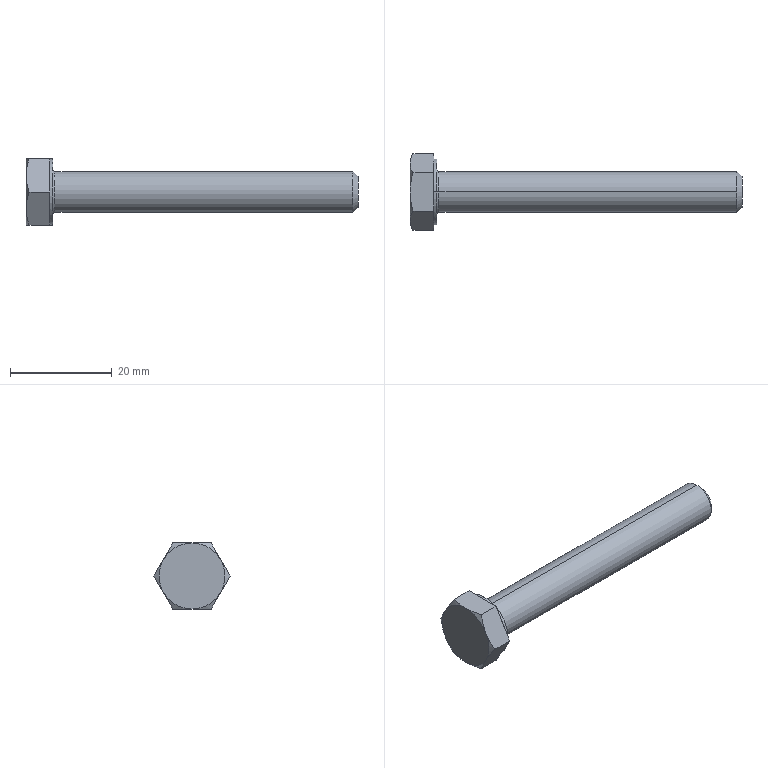Part | SolidWorks | features RevCut 4, Chamfer 1, Extrusion 1, Fillet 1, LPattern 1, Revolution 1 | 1 solid | 29 faces | box 65.3 x 15.011 x 13 mm | volume 3770 mm3 | plane 15 | cone 8 | cylinder 4 | torus 2 | commonest cylinder face diameters 8 x2 13 x2
STEP:
#1=CARTESIAN_POINT('',(5.7,0.,4.));
#2=VERTEX_POINT('',#1);
#3=CARTESIAN_POINT('',(5.7,0.,-4.));
#4=VERTEX_POINT('',#3);
#5=CARTESIAN_POINT('',(5.7,0.,0.));
#6=DIRECTION('',(1.,0.,0.));
#7=DIRECTION('',(0.,0.,-1.));
#8=AXIS2_PLACEMENT_3D('',#5,#6,#7);
#9=CIRCLE('',#8,4.);
#10=EDGE_CURVE('',#2,#4,#9,.T.);
#11=ORIENTED_EDGE('',*,*,#10,.F.);
#12=CARTESIAN_POINT('',(5.3,0.,4.4));
#13=VERTEX_POINT('',#12);
#14=CARTESIAN_POINT('',(5.7,0.,4.4));
#15=DIRECTION('',(0.,1.,0.));
#16=DIRECTION('',(0.,0.,1.));
#17=AXIS2_PLACEMENT_3D('',#14,#15,#16);
#18=CIRCLE('',#17,0.4);
#19=EDGE_CURVE('',#2,#13,#18,.T.);
#20=ORIENTED_EDGE('',*,*,#19,.T.);
#21=CARTESIAN_POINT('',(5.3,0.,-4.4));
#22=VERTEX_POINT('',#21);
#23=CARTESIAN_POINT('',(5.3,0.,0.));
#24=DIRECTION('',(-1.,0.,0.));
#25=DIRECTION('',(0.,0.,-1.));
#26=AXIS2_PLACEMENT_3D('',#23,#24,#25);
#27=CIRCLE('',#26,4.4);
#28=EDGE_CURVE('',#22,#13,#27,.T.);
#29=ORIENTED_EDGE('',*,*,#28,.F.);
#30=CARTESIAN_POINT('',(5.7,0.,-4.4));
#31=DIRECTION('',(0.,-1.,0.));
#32=DIRECTION('',(0.,0.,-1.));
#33=AXIS2_PLACEMENT_3D('',#30,#31,#32);
#34=CIRCLE('',#33,0.4);
#35=EDGE_CURVE('',#4,#22,#34,.T.);
#36=ORIENTED_EDGE('',*,*,#35,.F.);
#37=EDGE_LOOP('',(#11,#20,#29,#36));
#38=FACE_OUTER_BOUND('',#37,.T.);
#39=CARTESIAN_POINT('',(5.7,0.,0.));
#40=DIRECTION('',(1.,0.,0.));
#41=DIRECTION('',(0.,0.,-1.));
#42=AXIS2_PLACEMENT_3D('',#39,#40,#41);
#43=TOROIDAL_SURFACE('',#42,4.4,0.4);
#44=ADVANCED_FACE('',(#38),#43,.F.);
#45=CARTESIAN_POINT('',(65.3,0.,-3.));
#46=VERTEX_POINT('',#45);
#47=CARTESIAN_POINT('',(65.3,0.,3.));
#48=VERTEX_POINT('',#47);
#49=CARTESIAN_POINT('',(65.3,0.,0.));
#50=DIRECTION('',(1.,0.,0.));
#51=DIRECTION('',(0.,0.,1.));
#52=AXIS2_PLACEMENT_3D('',#49,#50,#51);
#53=CIRCLE('',#52,3.);
#54=EDGE_CURVE('',#46,#48,#53,.T.);
#55=ORIENTED_EDGE('',*,*,#54,.F.);
#56=CARTESIAN_POINT('',(64.3,0.,-4.));
#57=VERTEX_POINT('',#56);
#58=CARTESIAN_POINT('',(64.3,0.,-4.));
#59=DIRECTION('',(-0.7071,0.,-0.7071));
#60=VECTOR('',#59,1000.);
#61=LINE('',#58,#60);
#62=EDGE_CURVE('',#46,#57,#61,.T.);
#63=ORIENTED_EDGE('',*,*,#62,.T.);
#64=CARTESIAN_POINT('',(64.3,0.,4.));
#65=VERTEX_POINT('',#64);
#66=CARTESIAN_POINT('',(64.3,0.,0.));
#67=DIRECTION('',(-1.,0.,0.));
#68=DIRECTION('',(0.,0.,1.));
#69=AXIS2_PLACEMENT_3D('',#66,#67,#68);
#70=CIRCLE('',#69,4.);
#71=EDGE_CURVE('',#65,#57,#70,.T.);
#72=ORIENTED_EDGE('',*,*,#71,.F.);
#73=CARTESIAN_POINT('',(64.3,0.,4.));
#74=DIRECTION('',(-0.7071,0.,0.7071));
#75=VECTOR('',#74,1000.);
#76=LINE('',#73,#75);
#77=EDGE_CURVE('',#48,#65,#76,.T.);
#78=ORIENTED_EDGE('',*,*,#77,.F.);
#79=EDGE_LOOP('',(#55,#63,#72,#78));
#80=FACE_OUTER_BOUND('',#79,.T.);
#81=CARTESIAN_POINT('',(64.3,0.,0.));
#82=DIRECTION('',(-1.,0.,0.));
#83=DIRECTION('',(0.,0.,1.));
#84=AXIS2_PLACEMENT_3D('',#81,#82,#83);
#85=CONICAL_SURFACE('',#84,4.,0.7854);
#86=ADVANCED_FACE('',(#80),#85,.T.);
#87=ORIENTED_EDGE('',*,*,#71,.T.);
#88=CARTESIAN_POINT('',(0.,0.,-4.));
#89=DIRECTION('',(-1.,0.,0.));
#90=VECTOR('',#89,1000.);
#91=LINE('',#88,#90);
#92=EDGE_CURVE('',#57,#4,#91,.T.);
#93=ORIENTED_EDGE('',*,*,#92,.T.);
#94=CARTESIAN_POINT('',(5.7,0.,0.));
#95=DIRECTION('',(1.,0.,0.));
#96=DIRECTION('',(0.,0.,-1.));
#97=AXIS2_PLACEMENT_3D('',#94,#95,#96);
#98=CIRCLE('',#97,4.);
#99=EDGE_CURVE('',#4,#2,#98,.T.);
#100=ORIENTED_EDGE('',*,*,#99,.T.);
#101=CARTESIAN_POINT('',(0.,0.,4.));
#102=DIRECTION('',(-1.,0.,0.));
#103=VECTOR('',#102,1000.);
#104=LINE('',#101,#103);
#105=EDGE_CURVE('',#65,#2,#104,.T.);
#106=ORIENTED_EDGE('',*,*,#105,.F.);
#107=EDGE_LOOP('',(#87,#93,#100,#106));
#108=FACE_OUTER_BOUND('',#107,.T.);
#109=CARTESIAN_POINT('',(0.,0.,0.));
#110=DIRECTION('',(-1.,0.,0.));
#111=DIRECTION('',(0.,0.,1.));
#112=AXIS2_PLACEMENT_3D('',#109,#110,#111);
#113=CYLINDRICAL_SURFACE('',#112,4.);
#114=ADVANCED_FACE('',(#108),#113,.T.);
#115=CARTESIAN_POINT('',(5.3,0.,-6.5));
#116=VERTEX_POINT('',#115);
#117=CARTESIAN_POINT('',(5.3,0.,6.5));
#118=VERTEX_POINT('',#117);
#119=CARTESIAN_POINT('',(5.3,0.,0.));
#120=DIRECTION('',(1.,0.,0.));
#121=DIRECTION('',(0.,0.,-1.));
#122=AXIS2_PLACEMENT_3D('',#119,#120,#121);
#123=CIRCLE('',#122,6.5);
#124=EDGE_CURVE('',#116,#118,#123,.T.);
#125=ORIENTED_EDGE('',*,*,#124,.F.);
#126=CARTESIAN_POINT('',(4.7,0.,-6.5));
#127=VERTEX_POINT('',#126);
#128=CARTESIAN_POINT('',(0.,0.,-6.5));
#129=DIRECTION('',(-1.,0.,0.));
#130=VECTOR('',#129,1000.);
#131=LINE('',#128,#130);
#132=EDGE_CURVE('',#116,#127,#131,.T.);
#133=ORIENTED_EDGE('',*,*,#132,.T.);
#134=CARTESIAN_POINT('',(4.7,5.629,-3.25));
#135=VERTEX_POINT('',#134);
#136=CARTESIAN_POINT('',(4.7,0.,0.));
#137=DIRECTION('',(-1.,0.,0.));
#138=DIRECTION('',(0.,0.,1.));
#139=AXIS2_PLACEMENT_3D('',#136,#137,#138);
#140=CIRCLE('',#139,6.5);
#141=EDGE_CURVE('',#135,#127,#140,.T.);
#142=ORIENTED_EDGE('',*,*,#141,.F.);
#143=CARTESIAN_POINT('',(4.7,5.629,3.25));
#144=VERTEX_POINT('',#143);
#145=CARTESIAN_POINT('',(4.7,0.,0.));
#146=DIRECTION('',(-1.,0.,0.));
#147=DIRECTION('',(0.,0.,1.));
#148=AXIS2_PLACEMENT_3D('',#145,#146,#147);
#149=CIRCLE('',#148,6.5);
#150=EDGE_CURVE('',#144,#135,#149,.T.);
#151=ORIENTED_EDGE('',*,*,#150,.F.);
#152=CARTESIAN_POINT('',(4.7,0.,6.5));
#153=VERTEX_POINT('',#152);
#154=CARTESIAN_POINT('',(4.7,0.,0.));
#155=DIRECTION('',(-1.,0.,0.));
#156=DIRECTION('',(0.,0.,1.));
#157=AXIS2_PLACEMENT_3D('',#154,#155,#156);
#158=CIRCLE('',#157,6.5);
#159=EDGE_CURVE('',#153,#144,#158,.T.);
#160=ORIENTED_EDGE('',*,*,#159,.F.);
#161=CARTESIAN_POINT('',(0.,0.,6.5));
#162=DIRECTION('',(-1.,0.,0.));
#163=VECTOR('',#162,1000.);
#164=LINE('',#161,#163);
#165=EDGE_CURVE('',#118,#153,#164,.T.);
#166=ORIENTED_EDGE('',*,*,#165,.F.);
#167=EDGE_LOOP('',(#125,#133,#142,#151,#160,#166));
#168=FACE_OUTER_BOUND('',#167,.T.);
#169=CARTESIAN_POINT('',(0.,0.,0.));
#170=DIRECTION('',(-1.,0.,0.));
#171=DIRECTION('',(0.,0.,1.));
#172=AXIS2_PLACEMENT_3D('',#169,#170,#171);
#173=CYLINDRICAL_SURFACE('',#172,6.5);
#174=ADVANCED_FACE('',(#168),#173,.T.);
#175=CARTESIAN_POINT('',(4.7,3.753,-6.5));
#176=VERTEX_POINT('',#175);
#177=CARTESIAN_POINT('',(4.7,3.753,-6.5));
#178=DIRECTION('',(0.,0.5,0.866));
#179=VECTOR('',#178,1000.);
#180=LINE('',#177,#179);
#181=EDGE_CURVE('',#176,#135,#180,.T.);
#182=ORIENTED_EDGE('',*,*,#181,.F.);
#183=CARTESIAN_POINT('',(0.5806,3.753,-6.5));
#184=VERTEX_POINT('',#183);
#185=CARTESIAN_POINT('',(5.3,3.753,-6.5));
#186=DIRECTION('',(-1.,0.,0.));
#187=VECTOR('',#186,1000.);
#188=LINE('',#185,#187);
#189=EDGE_CURVE('',#176,#184,#188,.T.);
#190=ORIENTED_EDGE('',*,*,#189,.T.);
#191=CARTESIAN_POINT('',(0.,5.629,-3.25));
#192=VERTEX_POINT('',#191);
#193=CARTESIAN_POINT('',(0.,5.629,-3.25));
#194=CARTESIAN_POINT('',(0.,5.47,-3.526));
#195=CARTESIAN_POINT('',(0.01372,5.31,-3.803));
#196=CARTESIAN_POINT('',(0.06683,4.994,-4.351));
#197=CARTESIAN_POINT('',(0.1062,4.836,-4.623));
#198=CARTESIAN_POINT('',(0.2578,4.368,-5.435));
#199=CARTESIAN_POINT('',(0.4038,4.059,-5.97));
#200=CARTESIAN_POINT('',(0.5806,3.753,-6.5));
#201=B_SPLINE_CURVE_WITH_KNOTS('',3,(#193,#194,#195,#196,#197,#198,#199,#200),.UNSPECIFIED.,.F.,.F.,(4,2,2,4),(0.003797,0.004743,0.005689,0.00758),.UNSPECIFIED.);
#202=EDGE_CURVE('',#192,#184,#201,.T.);
#203=ORIENTED_EDGE('',*,*,#202,.F.);
#204=CARTESIAN_POINT('',(0.5806,7.506,0.));
#205=VERTEX_POINT('',#204);
#206=CARTESIAN_POINT('',(0.5806,7.506,0.));
#207=CARTESIAN_POINT('',(0.4033,7.199,-0.5317));
#208=CARTESIAN_POINT('',(0.2573,6.889,-1.067));
#209=CARTESIAN_POINT('',(0.05533,6.265,-2.149));
#210=CARTESIAN_POINT('',(0.,5.949,-2.696));
#211=CARTESIAN_POINT('',(0.,5.629,-3.25));
#212=B_SPLINE_CURVE_WITH_KNOTS('',3,(#206,#207,#208,#209,#210,#211),.UNSPECIFIED.,.F.,.F.,(4,2,4),(0.000000238,0.001899,0.003797),.UNSPECIFIED.);
#213=EDGE_CURVE('',#205,#192,#212,.T.);
#214=ORIENTED_EDGE('',*,*,#213,.F.);
#215=CARTESIAN_POINT('',(4.7,7.506,0.));
#216=VERTEX_POINT('',#215);
#217=CARTESIAN_POINT('',(5.3,7.506,0.));
#218=DIRECTION('',(-1.,0.,0.));
#219=VECTOR('',#218,1000.);
#220=LINE('',#217,#219);
#221=EDGE_CURVE('',#216,#205,#220,.T.);
#222=ORIENTED_EDGE('',*,*,#221,.F.);
#223=CARTESIAN_POINT('',(4.7,3.753,-6.5));
#224=DIRECTION('',(0.,0.5,0.866));
#225=VECTOR('',#224,1000.);
#226=LINE('',#223,#225);
#227=EDGE_CURVE('',#135,#216,#226,.T.);
#228=ORIENTED_EDGE('',*,*,#227,.F.);
#229=EDGE_LOOP('',(#182,#190,#203,#214,#222,#228));
#230=FACE_OUTER_BOUND('',#229,.T.);
#231=CARTESIAN_POINT('',(5.3,3.753,-6.5));
#232=DIRECTION('',(0.,-0.866,0.5));
#233=DIRECTION('',(0.,-0.5,-0.866));
#234=AXIS2_PLACEMENT_3D('',#231,#232,#233);
#235=PLANE('',#234);
#236=ADVANCED_FACE('',(#230),#235,.F.);
#237=CARTESIAN_POINT('',(4.7,7.506,0.));
#238=DIRECTION('',(0.,-0.5,0.866));
#239=VECTOR('',#238,1000.);
#240=LINE('',#237,#239);
#241=EDGE_CURVE('',#216,#144,#240,.T.);
#242=ORIENTED_EDGE('',*,*,#241,.F.);
#243=ORIENTED_EDGE('',*,*,#221,.T.);
#244=CARTESIAN_POINT('',(0.,5.629,3.25));
#245=VERTEX_POINT('',#244);
#246=CARTESIAN_POINT('',(0.,5.629,3.25));
#247=CARTESIAN_POINT('',(0.,5.788,2.974));
#248=CARTESIAN_POINT('',(0.01372,5.948,2.697));
#249=CARTESIAN_POINT('',(0.06683,6.265,2.149));
#250=CARTESIAN_POINT('',(0.1062,6.422,1.877));
#251=CARTESIAN_POINT('',(0.2578,6.891,1.065));
#252=CARTESIAN_POINT('',(0.4038,7.199,0.5303));
#253=CARTESIAN_POINT('',(0.5806,7.506,0.));
#254=B_SPLINE_CURVE_WITH_KNOTS('',3,(#246,#247,#248,#249,#250,#251,#252,#253),.UNSPECIFIED.,.F.,.F.,(4,2,2,4),(0.003797,0.004743,0.005689,0.00758),.UNSPECIFIED.);
#255=EDGE_CURVE('',#245,#205,#254,.T.);
#256=ORIENTED_EDGE('',*,*,#255,.F.);
#257=CARTESIAN_POINT('',(0.5806,3.753,6.5));
#258=VERTEX_POINT('',#257);
#259=CARTESIAN_POINT('',(0.5806,3.753,6.5));
#260=CARTESIAN_POINT('',(0.4033,4.06,5.968));
#261=CARTESIAN_POINT('',(0.2573,4.369,5.433));
#262=CARTESIAN_POINT('',(0.05533,4.994,4.351));
#263=CARTESIAN_POINT('',(0.,5.309,3.804));
#264=CARTESIAN_POINT('',(0.,5.629,3.25));
#265=B_SPLINE_CURVE_WITH_KNOTS('',3,(#259,#260,#261,#262,#263,#264),.UNSPECIFIED.,.F.,.F.,(4,2,4),(0.000000238,0.001899,0.003797),.UNSPECIFIED.);
#266=EDGE_CURVE('',#258,#245,#265,.T.);
#267=ORIENTED_EDGE('',*,*,#266,.F.);
#268=CARTESIAN_POINT('',(4.7,3.753,6.5));
#269=VERTEX_POINT('',#268);
#270=CARTESIAN_POINT('',(5.3,3.753,6.5));
#271=DIRECTION('',(-1.,0.,0.));
#272=VECTOR('',#271,1000.);
#273=LINE('',#270,#272);
#274=EDGE_CURVE('',#269,#258,#273,.T.);
#275=ORIENTED_EDGE('',*,*,#274,.F.);
#276=CARTESIAN_POINT('',(4.7,7.506,0.));
#277=DIRECTION('',(0.,-0.5,0.866));
#278=VECTOR('',#277,1000.);
#279=LINE('',#276,#278);
#280=EDGE_CURVE('',#144,#269,#279,.T.);
#281=ORIENTED_EDGE('',*,*,#280,.F.);
#282=EDGE_LOOP('',(#242,#243,#256,#267,#275,#281));
#283=FACE_OUTER_BOUND('',#282,.T.);
#284=CARTESIAN_POINT('',(5.3,7.506,0.));
#285=DIRECTION('',(0.,-0.866,-0.5));
#286=DIRECTION('',(0.,0.5,-0.866));
#287=AXIS2_PLACEMENT_3D('',#284,#285,#286);
#288=PLANE('',#287);
#289=ADVANCED_FACE('',(#283),#288,.F.);
#290=CARTESIAN_POINT('',(4.7,3.753,6.5));
#291=DIRECTION('',(0.,-1.,0.));
#292=VECTOR('',#291,1000.);
#293=LINE('',#290,#292);
#294=EDGE_CURVE('',#269,#153,#293,.T.);
#295=ORIENTED_EDGE('',*,*,#294,.F.);
#296=ORIENTED_EDGE('',*,*,#274,.T.);
#297=CARTESIAN_POINT('',(0.,0.,6.5));
#298=VERTEX_POINT('',#297);
#299=CARTESIAN_POINT('',(0.,0.,6.5));
#300=CARTESIAN_POINT('',(0.,0.6351,6.5));
#301=CARTESIAN_POINT('',(0.05613,1.279,6.5));
#302=CARTESIAN_POINT('',(0.2595,2.531,6.5));
#303=CARTESIAN_POINT('',(0.4054,3.146,6.5));
#304=CARTESIAN_POINT('',(0.5806,3.753,6.5));
#305=B_SPLINE_CURVE_WITH_KNOTS('',3,(#299,#300,#301,#302,#303,#304),.UNSPECIFIED.,.F.,.F.,(4,2,4),(0.01067,0.01257,0.01447),.UNSPECIFIED.);
#306=EDGE_CURVE('',#298,#258,#305,.T.);
#307=ORIENTED_EDGE('',*,*,#306,.F.);
#308=CARTESIAN_POINT('',(0.5806,-3.753,6.5));
#309=VERTEX_POINT('',#308);
#310=CARTESIAN_POINT('',(0.5806,-3.753,6.5));
#311=CARTESIAN_POINT('',(0.4042,-3.142,6.5));
#312=CARTESIAN_POINT('',(0.2565,-2.517,6.5));
#313=CARTESIAN_POINT('',(0.05459,-1.265,6.5));
#314=CARTESIAN_POINT('',(0.,-0.6347,6.5));
#315=CARTESIAN_POINT('',(0.,0.,6.5));
#316=B_SPLINE_CURVE_WITH_KNOTS('',3,(#310,#311,#312,#313,#314,#315),.UNSPECIFIED.,.F.,.F.,(4,2,4),(0.006874,0.008773,0.01067),.UNSPECIFIED.);
#317=EDGE_CURVE('',#309,#298,#316,.T.);
#318=ORIENTED_EDGE('',*,*,#317,.F.);
#319=CARTESIAN_POINT('',(4.7,-3.753,6.5));
#320=VERTEX_POINT('',#319);
#321=CARTESIAN_POINT('',(5.3,-3.753,6.5));
#322=DIRECTION('',(-1.,0.,0.));
#323=VECTOR('',#322,1000.);
#324=LINE('',#321,#323);
#325=EDGE_CURVE('',#320,#309,#324,.T.);
#326=ORIENTED_EDGE('',*,*,#325,.F.);
#327=CARTESIAN_POINT('',(4.7,3.753,6.5));
#328=DIRECTION('',(0.,-1.,0.));
#329=VECTOR('',#328,1000.);
#330=LINE('',#327,#329);
#331=EDGE_CURVE('',#153,#320,#330,.T.);
#332=ORIENTED_EDGE('',*,*,#331,.F.);
#333=EDGE_LOOP('',(#295,#296,#307,#318,#326,#332));
#334=FACE_OUTER_BOUND('',#333,.T.);
#335=CARTESIAN_POINT('',(5.3,3.753,6.5));
#336=DIRECTION('',(0.,0.,-1.));
#337=DIRECTION('',(0.,1.,0.));
#338=AXIS2_PLACEMENT_3D('',#335,#336,#337);
#339=PLANE('',#338);
#340=ADVANCED_FACE('',(#334),#339,.F.);
#341=CARTESIAN_POINT('',(4.7,-5.629,3.25));
#342=VERTEX_POINT('',#341);
#343=CARTESIAN_POINT('',(4.7,-7.506,0.));
#344=DIRECTION('',(0.,-0.5,-0.866));
#345=VECTOR('',#344,1000.);
#346=LINE('',#343,#345);
#347=EDGE_CURVE('',#320,#342,#346,.T.);
#348=ORIENTED_EDGE('',*,*,#347,.F.);
#349=ORIENTED_EDGE('',*,*,#325,.T.);
#350=CARTESIAN_POINT('',(0.,-5.629,3.25));
#351=VERTEX_POINT('',#350);
#352=CARTESIAN_POINT('',(0.,-5.629,3.25));
#353=CARTESIAN_POINT('',(0.,-5.47,3.526));
#354=CARTESIAN_POINT('',(0.01372,-5.31,3.803));
#355=CARTESIAN_POINT('',(0.06683,-4.994,4.351));
#356=CARTESIAN_POINT('',(0.1062,-4.836,4.623));
#357=CARTESIAN_POINT('',(0.2578,-4.368,5.435));
#358=CARTESIAN_POINT('',(0.4038,-4.059,5.97));
#359=CARTESIAN_POINT('',(0.5806,-3.753,6.5));
#360=B_SPLINE_CURVE_WITH_KNOTS('',3,(#352,#353,#354,#355,#356,#357,#358,#359),.UNSPECIFIED.,.F.,.F.,(4,2,2,4),(0.003797,0.004743,0.005689,0.00758),.UNSPECIFIED.);
#361=EDGE_CURVE('',#351,#309,#360,.T.);
#362=ORIENTED_EDGE('',*,*,#361,.F.);
#363=CARTESIAN_POINT('',(0.5806,-7.506,0.));
#364=VERTEX_POINT('',#363);
#365=CARTESIAN_POINT('',(0.5806,-7.506,0.));
#366=CARTESIAN_POINT('',(0.4033,-7.199,0.5317));
#367=CARTESIAN_POINT('',(0.2573,-6.889,1.067));
#368=CARTESIAN_POINT('',(0.05533,-6.265,2.149));
#369=CARTESIAN_POINT('',(0.,-5.949,2.696));
#370=CARTESIAN_POINT('',(0.,-5.629,3.25));
#371=B_SPLINE_CURVE_WITH_KNOTS('',3,(#365,#366,#367,#368,#369,#370),.UNSPECIFIED.,.F.,.F.,(4,2,4),(0.000000238,0.001899,0.003797),.UNSPECIFIED.);
#372=EDGE_CURVE('',#364,#351,#371,.T.);
#373=ORIENTED_EDGE('',*,*,#372,.F.);
#374=CARTESIAN_POINT('',(4.7,-7.506,0.));
#375=VERTEX_POINT('',#374);
#376=CARTESIAN_POINT('',(5.3,-7.506,0.));
#377=DIRECTION('',(-1.,0.,0.));
#378=VECTOR('',#377,1000.);
#379=LINE('',#376,#378);
#380=EDGE_CURVE('',#375,#364,#379,.T.);
#381=ORIENTED_EDGE('',*,*,#380,.F.);
#382=CARTESIAN_POINT('',(4.7,-7.506,0.));
#383=DIRECTION('',(0.,-0.5,-0.866));
#384=VECTOR('',#383,1000.);
#385=LINE('',#382,#384);
#386=EDGE_CURVE('',#342,#375,#385,.T.);
#387=ORIENTED_EDGE('',*,*,#386,.F.);
#388=EDGE_LOOP('',(#348,#349,#362,#373,#381,#387));
#389=FACE_OUTER_BOUND('',#388,.T.);
#390=CARTESIAN_POINT('',(5.3,-7.506,0.));
#391=DIRECTION('',(0.,0.866,-0.5));
#392=DIRECTION('',(0.,0.5,0.866));
#393=AXIS2_PLACEMENT_3D('',#390,#391,#392);
#394=PLANE('',#393);
#395=ADVANCED_FACE('',(#389),#394,.F.);
#396=CARTESIAN_POINT('',(4.7,-5.629,-3.25));
#397=VERTEX_POINT('',#396);
#398=CARTESIAN_POINT('',(4.7,-3.753,-6.5));
#399=DIRECTION('',(0.,0.5,-0.866));
#400=VECTOR('',#399,1000.);
#401=LINE('',#398,#400);
#402=EDGE_CURVE('',#375,#397,#401,.T.);
#403=ORIENTED_EDGE('',*,*,#402,.F.);
#404=ORIENTED_EDGE('',*,*,#380,.T.);
#405=CARTESIAN_POINT('',(0.,-5.629,-3.25));
#406=VERTEX_POINT('',#405);
#407=CARTESIAN_POINT('',(0.,-5.629,-3.25));
#408=CARTESIAN_POINT('',(0.,-5.788,-2.974));
#409=CARTESIAN_POINT('',(0.01372,-5.948,-2.697));
#410=CARTESIAN_POINT('',(0.06683,-6.265,-2.149));
#411=CARTESIAN_POINT('',(0.1062,-6.422,-1.877));
#412=CARTESIAN_POINT('',(0.2578,-6.891,-1.065));
#413=CARTESIAN_POINT('',(0.4038,-7.199,-0.5303));
#414=CARTESIAN_POINT('',(0.5806,-7.506,0.));
#415=B_SPLINE_CURVE_WITH_KNOTS('',3,(#407,#408,#409,#410,#411,#412,#413,#414),.UNSPECIFIED.,.F.,.F.,(4,2,2,4),(0.003797,0.004743,0.005689,0.00758),.UNSPECIFIED.);
#416=EDGE_CURVE('',#406,#364,#415,.T.);
#417=ORIENTED_EDGE('',*,*,#416,.F.);
#418=CARTESIAN_POINT('',(0.5806,-3.753,-6.5));
#419=VERTEX_POINT('',#418);
#420=CARTESIAN_POINT('',(0.5806,-3.753,-6.5));
#421=CARTESIAN_POINT('',(0.4033,-4.06,-5.968));
#422=CARTESIAN_POINT('',(0.2573,-4.369,-5.433));
#423=CARTESIAN_POINT('',(0.05533,-4.994,-4.351));
#424=CARTESIAN_POINT('',(0.,-5.309,-3.804));
#425=CARTESIAN_POINT('',(0.,-5.629,-3.25));
#426=B_SPLINE_CURVE_WITH_KNOTS('',3,(#420,#421,#422,#423,#424,#425),.UNSPECIFIED.,.F.,.F.,(4,2,4),(0.000000238,0.001899,0.003797),.UNSPECIFIED.);
#427=EDGE_CURVE('',#419,#406,#426,.T.);
#428=ORIENTED_EDGE('',*,*,#427,.F.);
#429=CARTESIAN_POINT('',(4.7,-3.753,-6.5));
#430=VERTEX_POINT('',#429);
#431=CARTESIAN_POINT('',(5.3,-3.753,-6.5));
#432=DIRECTION('',(-1.,0.,0.));
#433=VECTOR('',#432,1000.);
#434=LINE('',#431,#433);
#435=EDGE_CURVE('',#430,#419,#434,.T.);
#436=ORIENTED_EDGE('',*,*,#435,.F.);
#437=CARTESIAN_POINT('',(4.7,-3.753,-6.5));
#438=DIRECTION('',(0.,0.5,-0.866));
#439=VECTOR('',#438,1000.);
#440=LINE('',#437,#439);
#441=EDGE_CURVE('',#397,#430,#440,.T.);
#442=ORIENTED_EDGE('',*,*,#441,.F.);
#443=EDGE_LOOP('',(#403,#404,#417,#428,#436,#442));
#444=FACE_OUTER_BOUND('',#443,.T.);
#445=CARTESIAN_POINT('',(5.3,-3.753,-6.5));
#446=DIRECTION('',(0.,0.866,0.5));
#447=DIRECTION('',(0.,-0.5,0.866));
#448=AXIS2_PLACEMENT_3D('',#445,#446,#447);
#449=PLANE('',#448);
#450=ADVANCED_FACE('',(#444),#449,.F.);
#451=CARTESIAN_POINT('',(4.7,3.753,-6.5));
#452=DIRECTION('',(0.,1.,0.));
#453=VECTOR('',#452,1000.);
#454=LINE('',#451,#453);
#455=EDGE_CURVE('',#430,#127,#454,.T.);
#456=ORIENTED_EDGE('',*,*,#455,.F.);
#457=ORIENTED_EDGE('',*,*,#435,.T.);
#458=CARTESIAN_POINT('',(0.,0.,-6.5));
#459=VERTEX_POINT('',#458);
#460=CARTESIAN_POINT('',(0.,0.,-6.5));
#461=CARTESIAN_POINT('',(0.,-0.6347,-6.5));
#462=CARTESIAN_POINT('',(0.05459,-1.265,-6.5));
#463=CARTESIAN_POINT('',(0.2565,-2.517,-6.5));
#464=CARTESIAN_POINT('',(0.4042,-3.142,-6.5));
#465=CARTESIAN_POINT('',(0.5806,-3.753,-6.5));
#466=B_SPLINE_CURVE_WITH_KNOTS('',3,(#460,#461,#462,#463,#464,#465),.UNSPECIFIED.,.F.,.F.,(4,2,4),(0.02294,0.02484,0.02674),.UNSPECIFIED.);
#467=EDGE_CURVE('',#459,#419,#466,.T.);
#468=ORIENTED_EDGE('',*,*,#467,.F.);
#469=CARTESIAN_POINT('',(0.5806,3.753,-6.5));
#470=CARTESIAN_POINT('',(0.4054,3.146,-6.5));
#471=CARTESIAN_POINT('',(0.2595,2.531,-6.5));
#472=CARTESIAN_POINT('',(0.05613,1.279,-6.5));
#473=CARTESIAN_POINT('',(0.,0.6351,-6.5));
#474=CARTESIAN_POINT('',(0.,0.,-6.5));
#475=B_SPLINE_CURVE_WITH_KNOTS('',3,(#469,#470,#471,#472,#473,#474),.UNSPECIFIED.,.F.,.F.,(4,2,4),(0.01914,0.02104,0.02294),.UNSPECIFIED.);
#476=EDGE_CURVE('',#184,#459,#475,.T.);
#477=ORIENTED_EDGE('',*,*,#476,.F.);
#478=ORIENTED_EDGE('',*,*,#189,.F.);
#479=CARTESIAN_POINT('',(4.7,3.753,-6.5));
#480=DIRECTION('',(0.,1.,0.));
#481=VECTOR('',#480,1000.);
#482=LINE('',#479,#481);
#483=EDGE_CURVE('',#127,#176,#482,.T.);
#484=ORIENTED_EDGE('',*,*,#483,.F.);
#485=EDGE_LOOP('',(#456,#457,#468,#477,#478,#484));
#486=FACE_OUTER_BOUND('',#485,.T.);
#487=CARTESIAN_POINT('',(5.3,3.753,-6.5));
#488=DIRECTION('',(0.,0.,1.));
#489=DIRECTION('',(0.,-1.,0.));
#490=AXIS2_PLACEMENT_3D('',#487,#488,#489);
#491=PLANE('',#490);
#492=ADVANCED_FACE('',(#486),#491,.F.);
#493=ORIENTED_EDGE('',*,*,#427,.T.);
#494=CARTESIAN_POINT('',(0.,0.,0.));
#495=DIRECTION('',(1.,0.,0.));
#496=DIRECTION('',(0.,0.,-1.));
#497=AXIS2_PLACEMENT_3D('',#494,#495,#496);
#498=CIRCLE('',#497,6.5);
#499=EDGE_CURVE('',#406,#459,#498,.T.);
#500=ORIENTED_EDGE('',*,*,#499,.T.);
#501=ORIENTED_EDGE('',*,*,#467,.T.);
#502=EDGE_LOOP('',(#493,#500,#501));
#503=FACE_OUTER_BOUND('',#502,.T.);
#504=CARTESIAN_POINT('',(0.,0.,0.));
#505=DIRECTION('',(1.,0.,0.));
#506=DIRECTION('',(0.,0.,-1.));
#507=AXIS2_PLACEMENT_3D('',#504,#505,#506);
#508=CONICAL_SURFACE('',#507,6.5,1.047);
#509=ADVANCED_FACE('',(#503),#508,.T.);
#510=ORIENTED_EDGE('',*,*,#372,.T.);
#511=CARTESIAN_POINT('',(0.,0.,0.));
#512=DIRECTION('',(1.,0.,0.));
#513=DIRECTION('',(0.,0.,-1.));
#514=AXIS2_PLACEMENT_3D('',#511,#512,#513);
#515=CIRCLE('',#514,6.5);
#516=EDGE_CURVE('',#351,#406,#515,.T.);
#517=ORIENTED_EDGE('',*,*,#516,.T.);
#518=ORIENTED_EDGE('',*,*,#416,.T.);
#519=EDGE_LOOP('',(#510,#517,#518));
#520=FACE_OUTER_BOUND('',#519,.T.);
#521=CARTESIAN_POINT('',(0.,0.,0.));
#522=DIRECTION('',(1.,0.,0.));
#523=DIRECTION('',(0.,0.,-1.));
#524=AXIS2_PLACEMENT_3D('',#521,#522,#523);
#525=CONICAL_SURFACE('',#524,6.5,1.047);
#526=ADVANCED_FACE('',(#520),#525,.T.);
#527=ORIENTED_EDGE('',*,*,#317,.T.);
#528=CARTESIAN_POINT('',(0.,0.,0.));
#529=DIRECTION('',(1.,0.,0.));
#530=DIRECTION('',(0.,0.,-1.));
#531=AXIS2_PLACEMENT_3D('',#528,#529,#530);
#532=CIRCLE('',#531,6.5);
#533=EDGE_CURVE('',#298,#351,#532,.T.);
#534=ORIENTED_EDGE('',*,*,#533,.T.);
#535=ORIENTED_EDGE('',*,*,#361,.T.);
#536=EDGE_LOOP('',(#527,#534,#535));
#537=FACE_OUTER_BOUND('',#536,.T.);
#538=CARTESIAN_POINT('',(0.,0.,0.));
#539=DIRECTION('',(1.,0.,0.));
#540=DIRECTION('',(0.,0.,-1.));
#541=AXIS2_PLACEMENT_3D('',#538,#539,#540);
#542=CONICAL_SURFACE('',#541,6.5,1.047);
#543=ADVANCED_FACE('',(#537),#542,.T.);
#544=ORIENTED_EDGE('',*,*,#306,.T.);
#545=ORIENTED_EDGE('',*,*,#266,.T.);
#546=CARTESIAN_POINT('',(0.,0.,0.));
#547=DIRECTION('',(-1.,0.,0.));
#548=DIRECTION('',(0.,0.,1.));
#549=AXIS2_PLACEMENT_3D('',#546,#547,#548);
#550=CIRCLE('',#549,6.5);
#551=EDGE_CURVE('',#298,#245,#550,.T.);
#552=ORIENTED_EDGE('',*,*,#551,.F.);
#553=EDGE_LOOP('',(#544,#545,#552));
#554=FACE_OUTER_BOUND('',#553,.T.);
#555=CARTESIAN_POINT('',(0.,0.,0.));
#556=DIRECTION('',(1.,0.,0.));
#557=DIRECTION('',(0.,0.,-1.));
#558=AXIS2_PLACEMENT_3D('',#555,#556,#557);
#559=CONICAL_SURFACE('',#558,6.5,1.047);
#560=ADVANCED_FACE('',(#554),#559,.T.);
#561=ORIENTED_EDGE('',*,*,#255,.T.);
#562=ORIENTED_EDGE('',*,*,#213,.T.);
#563=CARTESIAN_POINT('',(0.,0.,0.));
#564=DIRECTION('',(1.,0.,0.));
#565=DIRECTION('',(0.,0.,-1.));
#566=AXIS2_PLACEMENT_3D('',#563,#564,#565);
#567=CIRCLE('',#566,6.5);
#568=EDGE_CURVE('',#192,#245,#567,.T.);
#569=ORIENTED_EDGE('',*,*,#568,.T.);
#570=EDGE_LOOP('',(#561,#562,#569));
#571=FACE_OUTER_BOUND('',#570,.T.);
#572=CARTESIAN_POINT('',(0.,0.,0.));
#573=DIRECTION('',(1.,0.,0.));
#574=DIRECTION('',(0.,0.,-1.));
#575=AXIS2_PLACEMENT_3D('',#572,#573,#574);
#576=CONICAL_SURFACE('',#575,6.5,1.047);
#577=ADVANCED_FACE('',(#571),#576,.T.);
#578=ORIENTED_EDGE('',*,*,#202,.T.);
#579=ORIENTED_EDGE('',*,*,#476,.T.);
#580=CARTESIAN_POINT('',(0.,0.,0.));
#581=DIRECTION('',(1.,0.,0.));
#582=DIRECTION('',(0.,0.,-1.));
#583=AXIS2_PLACEMENT_3D('',#580,#581,#582);
#584=CIRCLE('',#583,6.5);
#585=EDGE_CURVE('',#459,#192,#584,.T.);
#586=ORIENTED_EDGE('',*,*,#585,.T.);
#587=EDGE_LOOP('',(#578,#579,#586));
#588=FACE_OUTER_BOUND('',#587,.T.);
#589=CARTESIAN_POINT('',(0.,0.,0.));
#590=DIRECTION('',(1.,0.,0.));
#591=DIRECTION('',(0.,0.,-1.));
#592=AXIS2_PLACEMENT_3D('',#589,#590,#591);
#593=CONICAL_SURFACE('',#592,6.5,1.047);
#594=ADVANCED_FACE('',(#588),#593,.T.);
#595=ORIENTED_EDGE('',*,*,#585,.F.);
#596=ORIENTED_EDGE('',*,*,#499,.F.);
#597=ORIENTED_EDGE('',*,*,#516,.F.);
#598=ORIENTED_EDGE('',*,*,#533,.F.);
#599=ORIENTED_EDGE('',*,*,#551,.T.);
#600=ORIENTED_EDGE('',*,*,#568,.F.);
#601=EDGE_LOOP('',(#595,#596,#597,#598,#599,#600));
#602=FACE_OUTER_BOUND('',#601,.T.);
#603=CARTESIAN_POINT('',(0.,7.506,0.));
#604=DIRECTION('',(1.,0.,0.));
#605=DIRECTION('',(0.,0.,-1.));
#606=AXIS2_PLACEMENT_3D('',#603,#604,#605);
#607=PLANE('',#606);
#608=ADVANCED_FACE('',(#602),#607,.F.);
#609=ORIENTED_EDGE('',*,*,#181,.T.);
#610=ORIENTED_EDGE('',*,*,#141,.T.);
#611=ORIENTED_EDGE('',*,*,#483,.T.);
#612=EDGE_LOOP('',(#609,#610,#611));
#613=FACE_OUTER_BOUND('',#612,.T.);
#614=CARTESIAN_POINT('',(4.7,6.5,0.));
#615=DIRECTION('',(1.,0.,0.));
#616=DIRECTION('',(0.,0.,-1.));
#617=AXIS2_PLACEMENT_3D('',#614,#615,#616);
#618=PLANE('',#617);
#619=ADVANCED_FACE('',(#613),#618,.T.);
#620=ORIENTED_EDGE('',*,*,#227,.T.);
#621=ORIENTED_EDGE('',*,*,#241,.T.);
#622=ORIENTED_EDGE('',*,*,#150,.T.);
#623=EDGE_LOOP('',(#620,#621,#622));
#624=FACE_OUTER_BOUND('',#623,.T.);
#625=CARTESIAN_POINT('',(4.7,6.5,0.));
#626=DIRECTION('',(1.,0.,0.));
#627=DIRECTION('',(0.,0.,-1.));
#628=AXIS2_PLACEMENT_3D('',#625,#626,#627);
#629=PLANE('',#628);
#630=ADVANCED_FACE('',(#624),#629,.T.);
#631=ORIENTED_EDGE('',*,*,#280,.T.);
#632=ORIENTED_EDGE('',*,*,#294,.T.);
#633=ORIENTED_EDGE('',*,*,#159,.T.);
#634=EDGE_LOOP('',(#631,#632,#633));
#635=FACE_OUTER_BOUND('',#634,.T.);
#636=CARTESIAN_POINT('',(4.7,6.5,0.));
#637=DIRECTION('',(1.,0.,0.));
#638=DIRECTION('',(0.,0.,-1.));
#639=AXIS2_PLACEMENT_3D('',#636,#637,#638);
#640=PLANE('',#639);
#641=ADVANCED_FACE('',(#635),#640,.T.);
#642=ORIENTED_EDGE('',*,*,#331,.T.);
#643=ORIENTED_EDGE('',*,*,#347,.T.);
#644=CARTESIAN_POINT('',(4.7,0.,0.));
#645=DIRECTION('',(-1.,0.,0.));
#646=DIRECTION('',(0.,0.,1.));
#647=AXIS2_PLACEMENT_3D('',#644,#645,#646);
#648=CIRCLE('',#647,6.5);
#649=EDGE_CURVE('',#342,#153,#648,.T.);
#650=ORIENTED_EDGE('',*,*,#649,.T.);
#651=EDGE_LOOP('',(#642,#643,#650));
#652=FACE_OUTER_BOUND('',#651,.T.);
#653=CARTESIAN_POINT('',(4.7,6.5,0.));
#654=DIRECTION('',(1.,0.,0.));
#655=DIRECTION('',(0.,0.,-1.));
#656=AXIS2_PLACEMENT_3D('',#653,#654,#655);
#657=PLANE('',#656);
#658=ADVANCED_FACE('',(#652),#657,.T.);
#659=ORIENTED_EDGE('',*,*,#386,.T.);
#660=ORIENTED_EDGE('',*,*,#402,.T.);
#661=CARTESIAN_POINT('',(4.7,0.,0.));
#662=DIRECTION('',(-1.,0.,0.));
#663=DIRECTION('',(0.,0.,1.));
#664=AXIS2_PLACEMENT_3D('',#661,#662,#663);
#665=CIRCLE('',#664,6.5);
#666=EDGE_CURVE('',#397,#342,#665,.T.);
#667=ORIENTED_EDGE('',*,*,#666,.T.);
#668=EDGE_LOOP('',(#659,#660,#667));
#669=FACE_OUTER_BOUND('',#668,.T.);
#670=CARTESIAN_POINT('',(4.7,6.5,0.));
#671=DIRECTION('',(1.,0.,0.));
#672=DIRECTION('',(0.,0.,-1.));
#673=AXIS2_PLACEMENT_3D('',#670,#671,#672);
#674=PLANE('',#673);
#675=ADVANCED_FACE('',(#669),#674,.T.);
#676=ORIENTED_EDGE('',*,*,#441,.T.);
#677=ORIENTED_EDGE('',*,*,#455,.T.);
#678=CARTESIAN_POINT('',(4.7,0.,0.));
#679=DIRECTION('',(-1.,0.,0.));
#680=DIRECTION('',(0.,0.,1.));
#681=AXIS2_PLACEMENT_3D('',#678,#679,#680);
#682=CIRCLE('',#681,6.5);
#683=EDGE_CURVE('',#127,#397,#682,.T.);
#684=ORIENTED_EDGE('',*,*,#683,.T.);
#685=EDGE_LOOP('',(#676,#677,#684));
#686=FACE_OUTER_BOUND('',#685,.T.);
#687=CARTESIAN_POINT('',(4.7,6.5,0.));
#688=DIRECTION('',(1.,0.,0.));
#689=DIRECTION('',(0.,0.,-1.));
#690=AXIS2_PLACEMENT_3D('',#687,#688,#689);
#691=PLANE('',#690);
#692=ADVANCED_FACE('',(#686),#691,.T.);
#693=ORIENTED_EDGE('',*,*,#132,.F.);
#694=CARTESIAN_POINT('',(5.3,0.,0.));
#695=DIRECTION('',(1.,0.,0.));
#696=DIRECTION('',(0.,0.,-1.));
#697=AXIS2_PLACEMENT_3D('',#694,#695,#696);
#698=CIRCLE('',#697,6.5);
#699=EDGE_CURVE('',#118,#116,#698,.T.);
#700=ORIENTED_EDGE('',*,*,#699,.F.);
#701=ORIENTED_EDGE('',*,*,#165,.T.);
#702=ORIENTED_EDGE('',*,*,#649,.F.);
#703=ORIENTED_EDGE('',*,*,#666,.F.);
#704=ORIENTED_EDGE('',*,*,#683,.F.);
#705=EDGE_LOOP('',(#693,#700,#701,#702,#703,#704));
#706=FACE_OUTER_BOUND('',#705,.T.);
#707=CARTESIAN_POINT('',(0.,0.,0.));
#708=DIRECTION('',(-1.,0.,0.));
#709=DIRECTION('',(0.,0.,1.));
#710=AXIS2_PLACEMENT_3D('',#707,#708,#709);
#711=CYLINDRICAL_SURFACE('',#710,6.5);
#712=ADVANCED_FACE('',(#706),#711,.T.);
#713=CARTESIAN_POINT('',(65.3,0.,0.));
#714=DIRECTION('',(1.,0.,0.));
#715=DIRECTION('',(0.,0.,1.));
#716=AXIS2_PLACEMENT_3D('',#713,#714,#715);
#717=CIRCLE('',#716,3.);
#718=EDGE_CURVE('',#48,#46,#717,.T.);
#719=ORIENTED_EDGE('',*,*,#718,.T.);
#720=ORIENTED_EDGE('',*,*,#54,.T.);
#721=EDGE_LOOP('',(#719,#720));
#722=FACE_OUTER_BOUND('',#721,.T.);
#723=CARTESIAN_POINT('',(65.3,0.,0.));
#724=DIRECTION('',(-1.,0.,0.));
#725=DIRECTION('',(0.,0.,1.));
#726=AXIS2_PLACEMENT_3D('',#723,#724,#725);
#727=PLANE('',#726);
#728=ADVANCED_FACE('',(#722),#727,.F.);
#729=ORIENTED_EDGE('',*,*,#92,.F.);
#730=CARTESIAN_POINT('',(64.3,0.,0.));
#731=DIRECTION('',(-1.,0.,0.));
#732=DIRECTION('',(0.,0.,1.));
#733=AXIS2_PLACEMENT_3D('',#730,#731,#732);
#734=CIRCLE('',#733,4.);
#735=EDGE_CURVE('',#57,#65,#734,.T.);
#736=ORIENTED_EDGE('',*,*,#735,.T.);
#737=ORIENTED_EDGE('',*,*,#105,.T.);
#738=ORIENTED_EDGE('',*,*,#10,.T.);
#739=EDGE_LOOP('',(#729,#736,#737,#738));
#740=FACE_OUTER_BOUND('',#739,.T.);
#741=CARTESIAN_POINT('',(0.,0.,0.));
#742=DIRECTION('',(-1.,0.,0.));
#743=DIRECTION('',(0.,0.,1.));
#744=AXIS2_PLACEMENT_3D('',#741,#742,#743);
#745=CYLINDRICAL_SURFACE('',#744,4.);
#746=ADVANCED_FACE('',(#740),#745,.T.);
#747=ORIENTED_EDGE('',*,*,#28,.T.);
#748=CARTESIAN_POINT('',(5.3,0.,0.));
#749=DIRECTION('',(-1.,0.,0.));
#750=DIRECTION('',(0.,0.,-1.));
#751=AXIS2_PLACEMENT_3D('',#748,#749,#750);
#752=CIRCLE('',#751,4.4);
#753=EDGE_CURVE('',#13,#22,#752,.T.);
#754=ORIENTED_EDGE('',*,*,#753,.T.);
#755=EDGE_LOOP('',(#747,#754));
#756=FACE_BOUND('',#755,.T.);
#757=ORIENTED_EDGE('',*,*,#699,.T.);
#758=ORIENTED_EDGE('',*,*,#124,.T.);
#759=EDGE_LOOP('',(#757,#758));
#760=FACE_OUTER_BOUND('',#759,.T.);
#761=CARTESIAN_POINT('',(5.3,7.506,0.));
#762=DIRECTION('',(1.,0.,0.));
#763=DIRECTION('',(0.,0.,-1.));
#764=AXIS2_PLACEMENT_3D('',#761,#762,#763);
#765=PLANE('',#764);
#766=ADVANCED_FACE('',(#756,#760),#765,.T.);
#767=ORIENTED_EDGE('',*,*,#62,.F.);
#768=ORIENTED_EDGE('',*,*,#718,.F.);
#769=ORIENTED_EDGE('',*,*,#77,.T.);
#770=ORIENTED_EDGE('',*,*,#735,.F.);
#771=EDGE_LOOP('',(#767,#768,#769,#770));
#772=FACE_OUTER_BOUND('',#771,.T.);
#773=CARTESIAN_POINT('',(64.3,0.,0.));
#774=DIRECTION('',(-1.,0.,0.));
#775=DIRECTION('',(0.,0.,1.));
#776=AXIS2_PLACEMENT_3D('',#773,#774,#775);
#777=CONICAL_SURFACE('',#776,4.,0.7854);
#778=ADVANCED_FACE('',(#772),#777,.T.);
#779=ORIENTED_EDGE('',*,*,#19,.F.);
#780=ORIENTED_EDGE('',*,*,#99,.F.);
#781=ORIENTED_EDGE('',*,*,#35,.T.);
#782=ORIENTED_EDGE('',*,*,#753,.F.);
#783=EDGE_LOOP('',(#779,#780,#781,#782));
#784=FACE_OUTER_BOUND('',#783,.T.);
#785=CARTESIAN_POINT('',(5.7,0.,0.));
#786=DIRECTION('',(1.,0.,0.));
#787=DIRECTION('',(0.,0.,-1.));
#788=AXIS2_PLACEMENT_3D('',#785,#786,#787);
#789=TOROIDAL_SURFACE('',#788,4.4,0.4);
#790=ADVANCED_FACE('',(#784),#789,.F.);
#791=CLOSED_SHELL('',(#44,#86,#114,#174,#236,#289,#340,#395,#450,#492,#509,#526,#543,#560,#577,#594,#608,#619,#630,#641,#658,#675,#692,#712,#728,#746,#766,#778,#790));
#792=MANIFOLD_SOLID_BREP('',#791);
#793=CARTESIAN_POINT('',(0.,0.,0.));
#794=DIRECTION('',(0.,0.,1.));
#795=DIRECTION('',(1.,0.,0.));
#796=AXIS2_PLACEMENT_3D('',#793,#794,#795);
#797=(LENGTH_UNIT()NAMED_UNIT(*)SI_UNIT(.MILLI.,.METRE.));
#798=UNCERTAINTY_MEASURE_WITH_UNIT(LENGTH_MEASURE(0.00001),#797,'','');
#799=(NAMED_UNIT(*)PLANE_ANGLE_UNIT()SI_UNIT($,.RADIAN.));
#800=(NAMED_UNIT(*)SI_UNIT($,.STERADIAN.)SOLID_ANGLE_UNIT());
#801=(GEOMETRIC_REPRESENTATION_CONTEXT(3)GLOBAL_UNCERTAINTY_ASSIGNED_CONTEXT((#798))GLOBAL_UNIT_ASSIGNED_CONTEXT((#797,#799,#800))REPRESENTATION_CONTEXT('',''));
#802=ADVANCED_BREP_SHAPE_REPRESENTATION('',(#792,#796),#801);